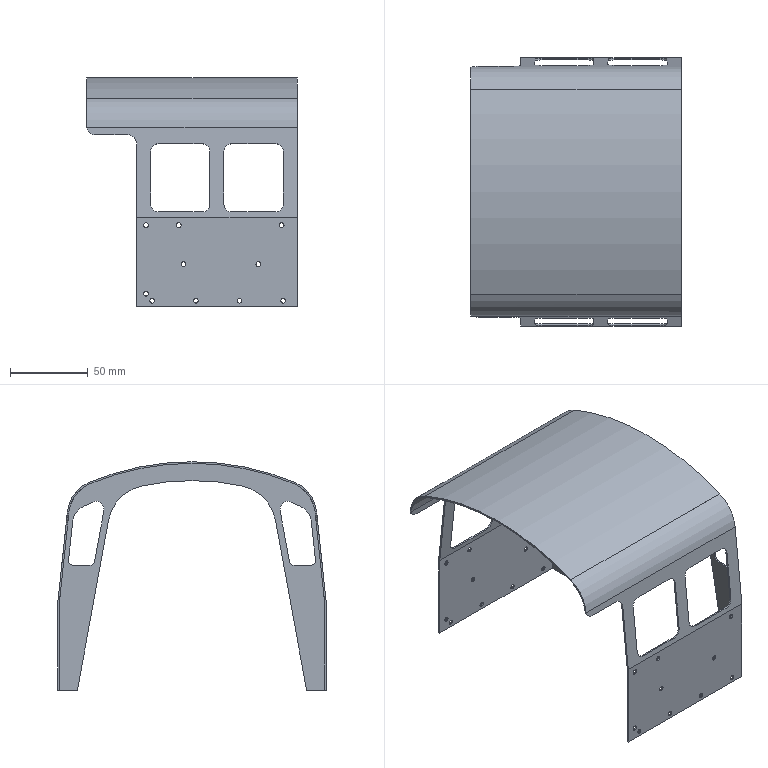Part | STEP file | 1-31.1 | 1 solid | 100 faces | box 135 x 172 x 146.5 mm | volume 47379 mm3 | cylinder 57 | plane 43 | commonest cylinder face diameters 3 x20 10 x18 6 x4 10.325 x2 12 x2 24 x2